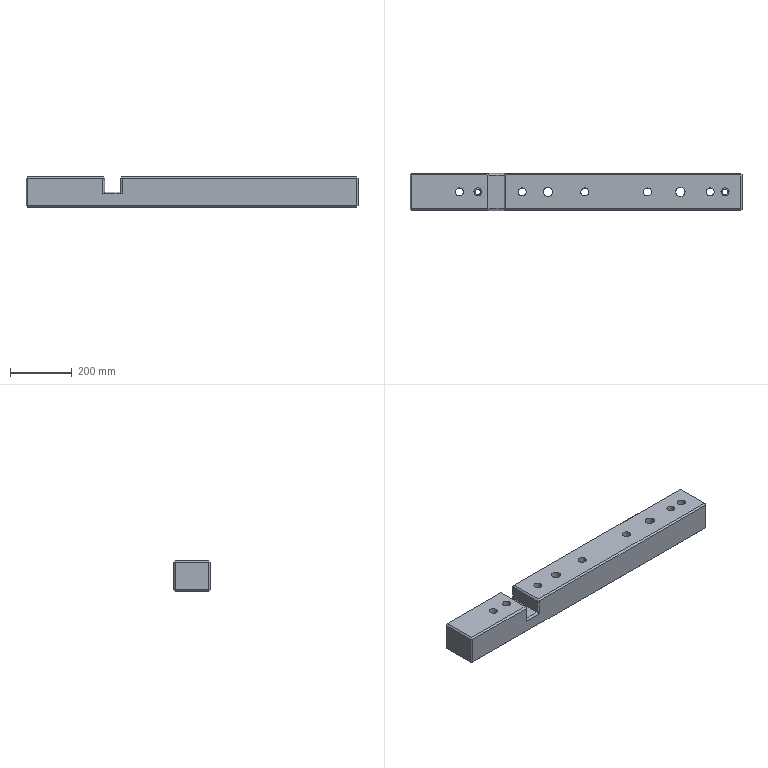Part | STEP file | solid 237 | 1 solid | 57 faces | box 1075 x 120 x 100 mm | volume 12067312 mm3 | plane 23 | spline 18 | cylinder 13 | other 3 | commonest cylinder face diameters 26 x7 12 x2 17.5 x2 30 x2